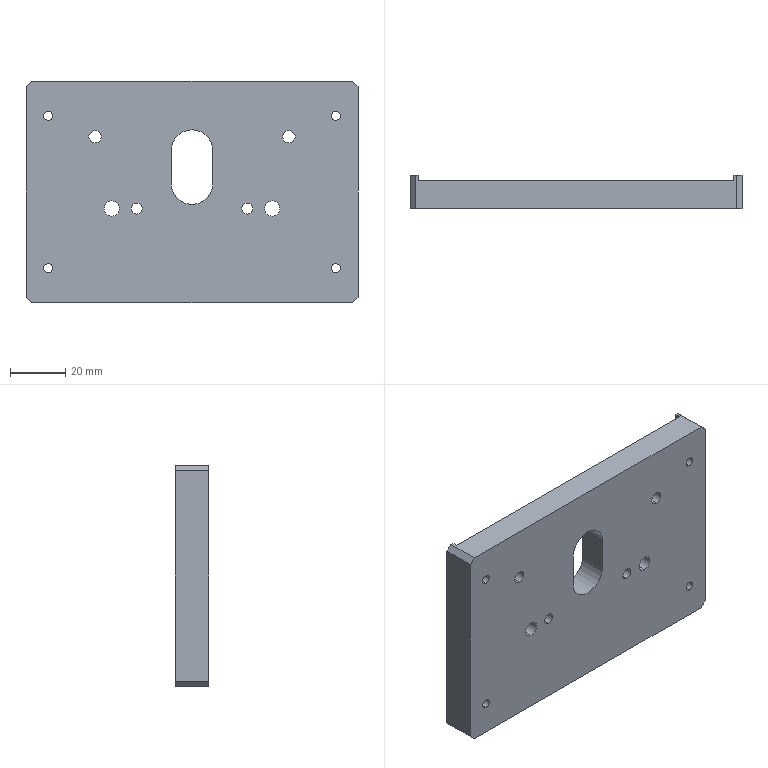Part | STEP file | PN_0030 | 1 solid | 51 faces | box 120 x 12 x 80 mm | volume 90970 mm3 | cylinder 31 | plane 20 | commonest cylinder face diameters 3.3 x8 4 x4 4.5 x4 5.5 x4 8 x4 10 x4